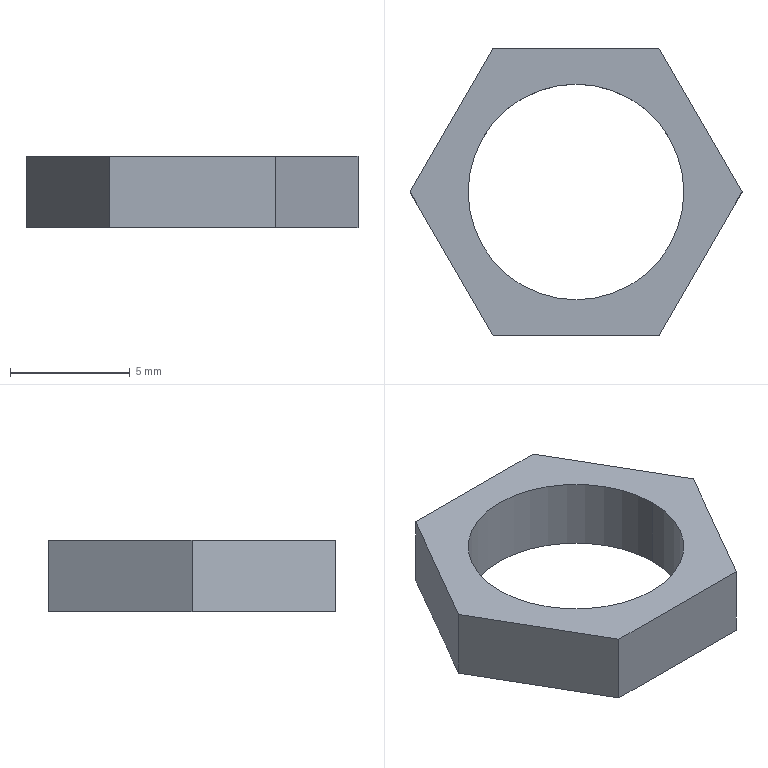Part | SolidWorks | features Extrusion 1, HoleWzd 1 | 1 solid | 10 faces | box 13.856 x 12 x 3 mm | volume 183.271 mm3 | plane 8 | cylinder 2 | commonest cylinder face diameters 9 x2
STEP:
#1=CARTESIAN_POINT('',(-4.5,0.,0.));
#2=VERTEX_POINT('',#1);
#3=CARTESIAN_POINT('',(4.5,0.,0.));
#4=VERTEX_POINT('',#3);
#5=CARTESIAN_POINT('',(0.,0.,0.));
#6=DIRECTION('',(0.,0.,1.));
#7=DIRECTION('',(1.,0.,0.));
#8=AXIS2_PLACEMENT_3D('',#5,#6,#7);
#9=CIRCLE('',#8,4.5);
#10=EDGE_CURVE('',#2,#4,#9,.T.);
#11=ORIENTED_EDGE('',*,*,#10,.F.);
#12=CARTESIAN_POINT('',(-4.5,0.,3.));
#13=VERTEX_POINT('',#12);
#14=CARTESIAN_POINT('',(-4.5,0.,3.));
#15=DIRECTION('',(0.,0.,1.));
#16=VECTOR('',#15,1000.);
#17=LINE('',#14,#16);
#18=EDGE_CURVE('',#2,#13,#17,.T.);
#19=ORIENTED_EDGE('',*,*,#18,.T.);
#20=CARTESIAN_POINT('',(4.5,0.,3.));
#21=VERTEX_POINT('',#20);
#22=CARTESIAN_POINT('',(0.,0.,3.));
#23=DIRECTION('',(0.,0.,1.));
#24=DIRECTION('',(1.,0.,0.));
#25=AXIS2_PLACEMENT_3D('',#22,#23,#24);
#26=CIRCLE('',#25,4.5);
#27=EDGE_CURVE('',#13,#21,#26,.T.);
#28=ORIENTED_EDGE('',*,*,#27,.T.);
#29=CARTESIAN_POINT('',(4.5,0.,3.));
#30=DIRECTION('',(0.,0.,1.));
#31=VECTOR('',#30,1000.);
#32=LINE('',#29,#31);
#33=EDGE_CURVE('',#4,#21,#32,.T.);
#34=ORIENTED_EDGE('',*,*,#33,.F.);
#35=EDGE_LOOP('',(#11,#19,#28,#34));
#36=FACE_OUTER_BOUND('',#35,.T.);
#37=CARTESIAN_POINT('',(0.,0.,3.));
#38=DIRECTION('',(0.,0.,1.));
#39=DIRECTION('',(1.,0.,0.));
#40=AXIS2_PLACEMENT_3D('',#37,#38,#39);
#41=CYLINDRICAL_SURFACE('',#40,4.5);
#42=ADVANCED_FACE('',(#36),#41,.F.);
#43=CARTESIAN_POINT('',(3.464,-6.,0.));
#44=VERTEX_POINT('',#43);
#45=CARTESIAN_POINT('',(6.928,0.,0.));
#46=VERTEX_POINT('',#45);
#47=CARTESIAN_POINT('',(3.464,-6.,0.));
#48=DIRECTION('',(0.5,0.866,0.));
#49=VECTOR('',#48,1000.);
#50=LINE('',#47,#49);
#51=EDGE_CURVE('',#44,#46,#50,.T.);
#52=ORIENTED_EDGE('',*,*,#51,.T.);
#53=CARTESIAN_POINT('',(6.928,0.,3.));
#54=VERTEX_POINT('',#53);
#55=CARTESIAN_POINT('',(6.928,0.,3.));
#56=DIRECTION('',(0.,0.,-1.));
#57=VECTOR('',#56,1000.);
#58=LINE('',#55,#57);
#59=EDGE_CURVE('',#54,#46,#58,.T.);
#60=ORIENTED_EDGE('',*,*,#59,.F.);
#61=CARTESIAN_POINT('',(3.464,-6.,3.));
#62=VERTEX_POINT('',#61);
#63=CARTESIAN_POINT('',(3.464,-6.,3.));
#64=DIRECTION('',(0.5,0.866,0.));
#65=VECTOR('',#64,1000.);
#66=LINE('',#63,#65);
#67=EDGE_CURVE('',#62,#54,#66,.T.);
#68=ORIENTED_EDGE('',*,*,#67,.F.);
#69=CARTESIAN_POINT('',(3.464,-6.,3.));
#70=DIRECTION('',(0.,0.,-1.));
#71=VECTOR('',#70,1000.);
#72=LINE('',#69,#71);
#73=EDGE_CURVE('',#62,#44,#72,.T.);
#74=ORIENTED_EDGE('',*,*,#73,.T.);
#75=EDGE_LOOP('',(#52,#60,#68,#74));
#76=FACE_OUTER_BOUND('',#75,.T.);
#77=CARTESIAN_POINT('',(3.464,-6.,3.));
#78=DIRECTION('',(-0.866,0.5,0.));
#79=DIRECTION('',(-0.5,-0.866,0.));
#80=AXIS2_PLACEMENT_3D('',#77,#78,#79);
#81=PLANE('',#80);
#82=ADVANCED_FACE('',(#76),#81,.F.);
#83=CARTESIAN_POINT('',(3.464,6.,0.));
#84=VERTEX_POINT('',#83);
#85=CARTESIAN_POINT('',(6.928,0.,0.));
#86=DIRECTION('',(-0.5,0.866,0.));
#87=VECTOR('',#86,1000.);
#88=LINE('',#85,#87);
#89=EDGE_CURVE('',#46,#84,#88,.T.);
#90=ORIENTED_EDGE('',*,*,#89,.T.);
#91=CARTESIAN_POINT('',(3.464,6.,3.));
#92=VERTEX_POINT('',#91);
#93=CARTESIAN_POINT('',(3.464,6.,3.));
#94=DIRECTION('',(0.,0.,-1.));
#95=VECTOR('',#94,1000.);
#96=LINE('',#93,#95);
#97=EDGE_CURVE('',#92,#84,#96,.T.);
#98=ORIENTED_EDGE('',*,*,#97,.F.);
#99=CARTESIAN_POINT('',(6.928,0.,3.));
#100=DIRECTION('',(-0.5,0.866,0.));
#101=VECTOR('',#100,1000.);
#102=LINE('',#99,#101);
#103=EDGE_CURVE('',#54,#92,#102,.T.);
#104=ORIENTED_EDGE('',*,*,#103,.F.);
#105=ORIENTED_EDGE('',*,*,#59,.T.);
#106=EDGE_LOOP('',(#90,#98,#104,#105));
#107=FACE_OUTER_BOUND('',#106,.T.);
#108=CARTESIAN_POINT('',(6.928,0.,3.));
#109=DIRECTION('',(-0.866,-0.5,0.));
#110=DIRECTION('',(0.5,-0.866,0.));
#111=AXIS2_PLACEMENT_3D('',#108,#109,#110);
#112=PLANE('',#111);
#113=ADVANCED_FACE('',(#107),#112,.F.);
#114=CARTESIAN_POINT('',(-3.464,6.,0.));
#115=VERTEX_POINT('',#114);
#116=CARTESIAN_POINT('',(3.464,6.,0.));
#117=DIRECTION('',(-1.,0.,0.));
#118=VECTOR('',#117,1000.);
#119=LINE('',#116,#118);
#120=EDGE_CURVE('',#84,#115,#119,.T.);
#121=ORIENTED_EDGE('',*,*,#120,.T.);
#122=CARTESIAN_POINT('',(-3.464,6.,3.));
#123=VERTEX_POINT('',#122);
#124=CARTESIAN_POINT('',(-3.464,6.,3.));
#125=DIRECTION('',(0.,0.,-1.));
#126=VECTOR('',#125,1000.);
#127=LINE('',#124,#126);
#128=EDGE_CURVE('',#123,#115,#127,.T.);
#129=ORIENTED_EDGE('',*,*,#128,.F.);
#130=CARTESIAN_POINT('',(3.464,6.,3.));
#131=DIRECTION('',(-1.,0.,0.));
#132=VECTOR('',#131,1000.);
#133=LINE('',#130,#132);
#134=EDGE_CURVE('',#92,#123,#133,.T.);
#135=ORIENTED_EDGE('',*,*,#134,.F.);
#136=ORIENTED_EDGE('',*,*,#97,.T.);
#137=EDGE_LOOP('',(#121,#129,#135,#136));
#138=FACE_OUTER_BOUND('',#137,.T.);
#139=CARTESIAN_POINT('',(3.464,6.,3.));
#140=DIRECTION('',(0.,-1.,0.));
#141=DIRECTION('',(1.,0.,0.));
#142=AXIS2_PLACEMENT_3D('',#139,#140,#141);
#143=PLANE('',#142);
#144=ADVANCED_FACE('',(#138),#143,.F.);
#145=CARTESIAN_POINT('',(-6.928,0.,0.));
#146=VERTEX_POINT('',#145);
#147=CARTESIAN_POINT('',(-3.464,6.,0.));
#148=DIRECTION('',(-0.5,-0.866,0.));
#149=VECTOR('',#148,1000.);
#150=LINE('',#147,#149);
#151=EDGE_CURVE('',#115,#146,#150,.T.);
#152=ORIENTED_EDGE('',*,*,#151,.T.);
#153=CARTESIAN_POINT('',(-6.928,0.,3.));
#154=VERTEX_POINT('',#153);
#155=CARTESIAN_POINT('',(-6.928,0.,3.));
#156=DIRECTION('',(0.,0.,-1.));
#157=VECTOR('',#156,1000.);
#158=LINE('',#155,#157);
#159=EDGE_CURVE('',#154,#146,#158,.T.);
#160=ORIENTED_EDGE('',*,*,#159,.F.);
#161=CARTESIAN_POINT('',(-3.464,6.,3.));
#162=DIRECTION('',(-0.5,-0.866,0.));
#163=VECTOR('',#162,1000.);
#164=LINE('',#161,#163);
#165=EDGE_CURVE('',#123,#154,#164,.T.);
#166=ORIENTED_EDGE('',*,*,#165,.F.);
#167=ORIENTED_EDGE('',*,*,#128,.T.);
#168=EDGE_LOOP('',(#152,#160,#166,#167));
#169=FACE_OUTER_BOUND('',#168,.T.);
#170=CARTESIAN_POINT('',(-3.464,6.,3.));
#171=DIRECTION('',(0.866,-0.5,0.));
#172=DIRECTION('',(0.5,0.866,0.));
#173=AXIS2_PLACEMENT_3D('',#170,#171,#172);
#174=PLANE('',#173);
#175=ADVANCED_FACE('',(#169),#174,.F.);
#176=CARTESIAN_POINT('',(-3.464,-6.,0.));
#177=VERTEX_POINT('',#176);
#178=CARTESIAN_POINT('',(-6.928,0.,0.));
#179=DIRECTION('',(0.5,-0.866,0.));
#180=VECTOR('',#179,1000.);
#181=LINE('',#178,#180);
#182=EDGE_CURVE('',#146,#177,#181,.T.);
#183=ORIENTED_EDGE('',*,*,#182,.T.);
#184=CARTESIAN_POINT('',(-3.464,-6.,3.));
#185=VERTEX_POINT('',#184);
#186=CARTESIAN_POINT('',(-3.464,-6.,3.));
#187=DIRECTION('',(0.,0.,-1.));
#188=VECTOR('',#187,1000.);
#189=LINE('',#186,#188);
#190=EDGE_CURVE('',#185,#177,#189,.T.);
#191=ORIENTED_EDGE('',*,*,#190,.F.);
#192=CARTESIAN_POINT('',(-6.928,0.,3.));
#193=DIRECTION('',(0.5,-0.866,0.));
#194=VECTOR('',#193,1000.);
#195=LINE('',#192,#194);
#196=EDGE_CURVE('',#154,#185,#195,.T.);
#197=ORIENTED_EDGE('',*,*,#196,.F.);
#198=ORIENTED_EDGE('',*,*,#159,.T.);
#199=EDGE_LOOP('',(#183,#191,#197,#198));
#200=FACE_OUTER_BOUND('',#199,.T.);
#201=CARTESIAN_POINT('',(-6.928,0.,3.));
#202=DIRECTION('',(0.866,0.5,0.));
#203=DIRECTION('',(-0.5,0.866,0.));
#204=AXIS2_PLACEMENT_3D('',#201,#202,#203);
#205=PLANE('',#204);
#206=ADVANCED_FACE('',(#200),#205,.F.);
#207=CARTESIAN_POINT('',(-3.464,-6.,0.));
#208=DIRECTION('',(1.,0.,0.));
#209=VECTOR('',#208,1000.);
#210=LINE('',#207,#209);
#211=EDGE_CURVE('',#177,#44,#210,.T.);
#212=ORIENTED_EDGE('',*,*,#211,.T.);
#213=ORIENTED_EDGE('',*,*,#73,.F.);
#214=CARTESIAN_POINT('',(-3.464,-6.,3.));
#215=DIRECTION('',(1.,0.,0.));
#216=VECTOR('',#215,1000.);
#217=LINE('',#214,#216);
#218=EDGE_CURVE('',#185,#62,#217,.T.);
#219=ORIENTED_EDGE('',*,*,#218,.F.);
#220=ORIENTED_EDGE('',*,*,#190,.T.);
#221=EDGE_LOOP('',(#212,#213,#219,#220));
#222=FACE_OUTER_BOUND('',#221,.T.);
#223=CARTESIAN_POINT('',(-3.464,-6.,3.));
#224=DIRECTION('',(0.,1.,0.));
#225=DIRECTION('',(-1.,0.,0.));
#226=AXIS2_PLACEMENT_3D('',#223,#224,#225);
#227=PLANE('',#226);
#228=ADVANCED_FACE('',(#222),#227,.F.);
#229=CARTESIAN_POINT('',(0.,0.,3.));
#230=DIRECTION('',(0.,0.,1.));
#231=DIRECTION('',(1.,0.,0.));
#232=AXIS2_PLACEMENT_3D('',#229,#230,#231);
#233=CIRCLE('',#232,4.5);
#234=EDGE_CURVE('',#21,#13,#233,.T.);
#235=ORIENTED_EDGE('',*,*,#234,.F.);
#236=ORIENTED_EDGE('',*,*,#27,.F.);
#237=EDGE_LOOP('',(#235,#236));
#238=FACE_BOUND('',#237,.T.);
#239=ORIENTED_EDGE('',*,*,#67,.T.);
#240=ORIENTED_EDGE('',*,*,#103,.T.);
#241=ORIENTED_EDGE('',*,*,#134,.T.);
#242=ORIENTED_EDGE('',*,*,#165,.T.);
#243=ORIENTED_EDGE('',*,*,#196,.T.);
#244=ORIENTED_EDGE('',*,*,#218,.T.);
#245=EDGE_LOOP('',(#239,#240,#241,#242,#243,#244));
#246=FACE_OUTER_BOUND('',#245,.T.);
#247=CARTESIAN_POINT('',(0.,0.,3.));
#248=DIRECTION('',(0.,0.,1.));
#249=DIRECTION('',(1.,0.,0.));
#250=AXIS2_PLACEMENT_3D('',#247,#248,#249);
#251=PLANE('',#250);
#252=ADVANCED_FACE('',(#238,#246),#251,.T.);
#253=CARTESIAN_POINT('',(0.,0.,0.));
#254=DIRECTION('',(0.,0.,1.));
#255=DIRECTION('',(1.,0.,0.));
#256=AXIS2_PLACEMENT_3D('',#253,#254,#255);
#257=CIRCLE('',#256,4.5);
#258=EDGE_CURVE('',#4,#2,#257,.T.);
#259=ORIENTED_EDGE('',*,*,#258,.T.);
#260=ORIENTED_EDGE('',*,*,#10,.T.);
#261=EDGE_LOOP('',(#259,#260));
#262=FACE_BOUND('',#261,.T.);
#263=ORIENTED_EDGE('',*,*,#51,.F.);
#264=ORIENTED_EDGE('',*,*,#211,.F.);
#265=ORIENTED_EDGE('',*,*,#182,.F.);
#266=ORIENTED_EDGE('',*,*,#151,.F.);
#267=ORIENTED_EDGE('',*,*,#120,.F.);
#268=ORIENTED_EDGE('',*,*,#89,.F.);
#269=EDGE_LOOP('',(#263,#264,#265,#266,#267,#268));
#270=FACE_OUTER_BOUND('',#269,.T.);
#271=CARTESIAN_POINT('',(0.,0.,0.));
#272=DIRECTION('',(0.,0.,1.));
#273=DIRECTION('',(1.,0.,0.));
#274=AXIS2_PLACEMENT_3D('',#271,#272,#273);
#275=PLANE('',#274);
#276=ADVANCED_FACE('',(#262,#270),#275,.F.);
#277=ORIENTED_EDGE('',*,*,#18,.F.);
#278=ORIENTED_EDGE('',*,*,#258,.F.);
#279=ORIENTED_EDGE('',*,*,#33,.T.);
#280=ORIENTED_EDGE('',*,*,#234,.T.);
#281=EDGE_LOOP('',(#277,#278,#279,#280));
#282=FACE_OUTER_BOUND('',#281,.T.);
#283=CARTESIAN_POINT('',(0.,0.,3.));
#284=DIRECTION('',(0.,0.,1.));
#285=DIRECTION('',(1.,0.,0.));
#286=AXIS2_PLACEMENT_3D('',#283,#284,#285);
#287=CYLINDRICAL_SURFACE('',#286,4.5);
#288=ADVANCED_FACE('',(#282),#287,.F.);
#289=CLOSED_SHELL('',(#42,#82,#113,#144,#175,#206,#228,#252,#276,#288));
#290=MANIFOLD_SOLID_BREP('',#289);
#291=CARTESIAN_POINT('',(0.,0.,0.));
#292=DIRECTION('',(0.,0.,1.));
#293=DIRECTION('',(1.,0.,0.));
#294=AXIS2_PLACEMENT_3D('',#291,#292,#293);
#295=(LENGTH_UNIT()NAMED_UNIT(*)SI_UNIT(.MILLI.,.METRE.));
#296=UNCERTAINTY_MEASURE_WITH_UNIT(LENGTH_MEASURE(0.00001),#295,'','');
#297=(NAMED_UNIT(*)PLANE_ANGLE_UNIT()SI_UNIT($,.RADIAN.));
#298=(NAMED_UNIT(*)SI_UNIT($,.STERADIAN.)SOLID_ANGLE_UNIT());
#299=(GEOMETRIC_REPRESENTATION_CONTEXT(3)GLOBAL_UNCERTAINTY_ASSIGNED_CONTEXT((#296))GLOBAL_UNIT_ASSIGNED_CONTEXT((#295,#297,#298))REPRESENTATION_CONTEXT('',''));
#300=ADVANCED_BREP_SHAPE_REPRESENTATION('',(#290,#294),#299);